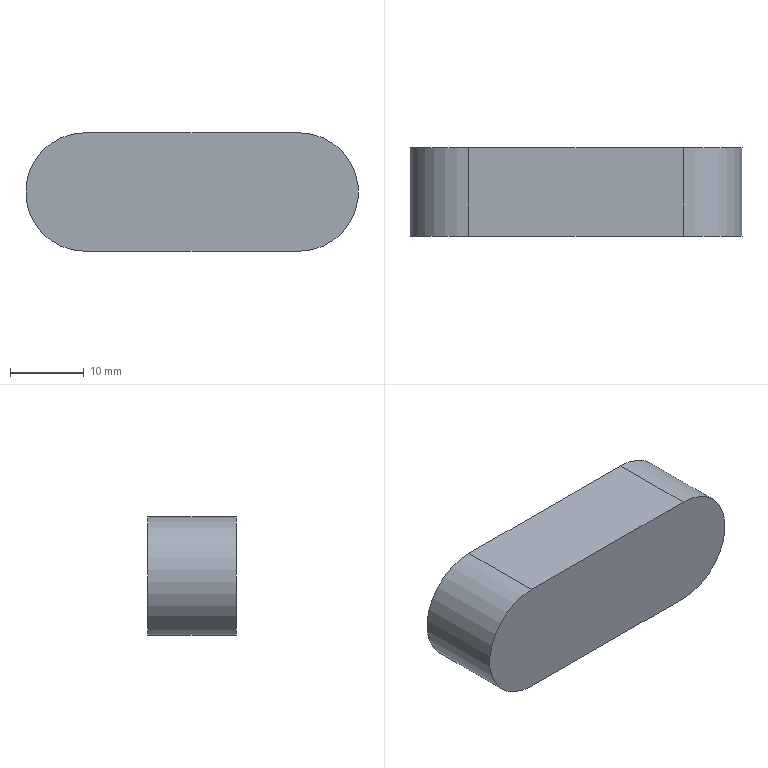Part | SolidWorks | features Extrusion 1 | 1 solid | 6 faces | box 45 x 12 x 16 mm | volume 7981 mm3 | plane 4 | cylinder 2 | commonest cylinder face diameters 16 x2
STEP:
#1=CARTESIAN_POINT('',(0.,0.,-8.));
#2=VERTEX_POINT('',#1);
#3=CARTESIAN_POINT('',(0.,0.,8.));
#4=VERTEX_POINT('',#3);
#5=CARTESIAN_POINT('',(0.,0.,0.));
#6=DIRECTION('',(0.,1.,0.));
#7=DIRECTION('',(0.,0.,1.));
#8=AXIS2_PLACEMENT_3D('',#5,#6,#7);
#9=CIRCLE('',#8,8.);
#10=EDGE_CURVE('',#2,#4,#9,.T.);
#11=ORIENTED_EDGE('',*,*,#10,.T.);
#12=CARTESIAN_POINT('',(0.,12.,8.));
#13=VERTEX_POINT('',#12);
#14=CARTESIAN_POINT('',(0.,12.,8.));
#15=DIRECTION('',(0.,-1.,0.));
#16=VECTOR('',#15,1000.);
#17=LINE('',#14,#16);
#18=EDGE_CURVE('',#13,#4,#17,.T.);
#19=ORIENTED_EDGE('',*,*,#18,.F.);
#20=CARTESIAN_POINT('',(0.,12.,-8.));
#21=VERTEX_POINT('',#20);
#22=CARTESIAN_POINT('',(0.,12.,0.));
#23=DIRECTION('',(0.,1.,0.));
#24=DIRECTION('',(0.,0.,1.));
#25=AXIS2_PLACEMENT_3D('',#22,#23,#24);
#26=CIRCLE('',#25,8.);
#27=EDGE_CURVE('',#21,#13,#26,.T.);
#28=ORIENTED_EDGE('',*,*,#27,.F.);
#29=CARTESIAN_POINT('',(0.,12.,-8.));
#30=DIRECTION('',(0.,-1.,0.));
#31=VECTOR('',#30,1000.);
#32=LINE('',#29,#31);
#33=EDGE_CURVE('',#21,#2,#32,.T.);
#34=ORIENTED_EDGE('',*,*,#33,.T.);
#35=EDGE_LOOP('',(#11,#19,#28,#34));
#36=FACE_OUTER_BOUND('',#35,.T.);
#37=CARTESIAN_POINT('',(0.,12.,0.));
#38=DIRECTION('',(0.,-1.,0.));
#39=DIRECTION('',(0.,0.,-1.));
#40=AXIS2_PLACEMENT_3D('',#37,#38,#39);
#41=CYLINDRICAL_SURFACE('',#40,8.);
#42=ADVANCED_FACE('',(#36),#41,.T.);
#43=CARTESIAN_POINT('',(29.,0.,8.));
#44=VERTEX_POINT('',#43);
#45=CARTESIAN_POINT('',(0.,0.,8.));
#46=DIRECTION('',(1.,0.,0.));
#47=VECTOR('',#46,1000.);
#48=LINE('',#45,#47);
#49=EDGE_CURVE('',#4,#44,#48,.T.);
#50=ORIENTED_EDGE('',*,*,#49,.T.);
#51=CARTESIAN_POINT('',(29.,12.,8.));
#52=VERTEX_POINT('',#51);
#53=CARTESIAN_POINT('',(29.,12.,8.));
#54=DIRECTION('',(0.,-1.,0.));
#55=VECTOR('',#54,1000.);
#56=LINE('',#53,#55);
#57=EDGE_CURVE('',#52,#44,#56,.T.);
#58=ORIENTED_EDGE('',*,*,#57,.F.);
#59=CARTESIAN_POINT('',(0.,12.,8.));
#60=DIRECTION('',(1.,0.,0.));
#61=VECTOR('',#60,1000.);
#62=LINE('',#59,#61);
#63=EDGE_CURVE('',#13,#52,#62,.T.);
#64=ORIENTED_EDGE('',*,*,#63,.F.);
#65=ORIENTED_EDGE('',*,*,#18,.T.);
#66=EDGE_LOOP('',(#50,#58,#64,#65));
#67=FACE_OUTER_BOUND('',#66,.T.);
#68=CARTESIAN_POINT('',(0.,12.,8.));
#69=DIRECTION('',(0.,0.,-1.));
#70=DIRECTION('',(-1.,0.,0.));
#71=AXIS2_PLACEMENT_3D('',#68,#69,#70);
#72=PLANE('',#71);
#73=ADVANCED_FACE('',(#67),#72,.F.);
#74=CARTESIAN_POINT('',(29.,0.,-8.));
#75=VERTEX_POINT('',#74);
#76=CARTESIAN_POINT('',(29.,0.,0.));
#77=DIRECTION('',(0.,1.,0.));
#78=DIRECTION('',(0.,0.,1.));
#79=AXIS2_PLACEMENT_3D('',#76,#77,#78);
#80=CIRCLE('',#79,8.);
#81=EDGE_CURVE('',#44,#75,#80,.T.);
#82=ORIENTED_EDGE('',*,*,#81,.T.);
#83=CARTESIAN_POINT('',(29.,12.,-8.));
#84=VERTEX_POINT('',#83);
#85=CARTESIAN_POINT('',(29.,12.,-8.));
#86=DIRECTION('',(0.,-1.,0.));
#87=VECTOR('',#86,1000.);
#88=LINE('',#85,#87);
#89=EDGE_CURVE('',#84,#75,#88,.T.);
#90=ORIENTED_EDGE('',*,*,#89,.F.);
#91=CARTESIAN_POINT('',(29.,12.,0.));
#92=DIRECTION('',(0.,1.,0.));
#93=DIRECTION('',(0.,0.,1.));
#94=AXIS2_PLACEMENT_3D('',#91,#92,#93);
#95=CIRCLE('',#94,8.);
#96=EDGE_CURVE('',#52,#84,#95,.T.);
#97=ORIENTED_EDGE('',*,*,#96,.F.);
#98=ORIENTED_EDGE('',*,*,#57,.T.);
#99=EDGE_LOOP('',(#82,#90,#97,#98));
#100=FACE_OUTER_BOUND('',#99,.T.);
#101=CARTESIAN_POINT('',(29.,12.,0.));
#102=DIRECTION('',(0.,-1.,0.));
#103=DIRECTION('',(0.,0.,-1.));
#104=AXIS2_PLACEMENT_3D('',#101,#102,#103);
#105=CYLINDRICAL_SURFACE('',#104,8.);
#106=ADVANCED_FACE('',(#100),#105,.T.);
#107=CARTESIAN_POINT('',(0.,0.,-8.));
#108=DIRECTION('',(-1.,0.,0.));
#109=VECTOR('',#108,1000.);
#110=LINE('',#107,#109);
#111=EDGE_CURVE('',#75,#2,#110,.T.);
#112=ORIENTED_EDGE('',*,*,#111,.T.);
#113=ORIENTED_EDGE('',*,*,#33,.F.);
#114=CARTESIAN_POINT('',(0.,12.,-8.));
#115=DIRECTION('',(-1.,0.,0.));
#116=VECTOR('',#115,1000.);
#117=LINE('',#114,#116);
#118=EDGE_CURVE('',#84,#21,#117,.T.);
#119=ORIENTED_EDGE('',*,*,#118,.F.);
#120=ORIENTED_EDGE('',*,*,#89,.T.);
#121=EDGE_LOOP('',(#112,#113,#119,#120));
#122=FACE_OUTER_BOUND('',#121,.T.);
#123=CARTESIAN_POINT('',(0.,12.,-8.));
#124=DIRECTION('',(0.,0.,1.));
#125=DIRECTION('',(1.,0.,0.));
#126=AXIS2_PLACEMENT_3D('',#123,#124,#125);
#127=PLANE('',#126);
#128=ADVANCED_FACE('',(#122),#127,.F.);
#129=ORIENTED_EDGE('',*,*,#27,.T.);
#130=ORIENTED_EDGE('',*,*,#63,.T.);
#131=ORIENTED_EDGE('',*,*,#96,.T.);
#132=ORIENTED_EDGE('',*,*,#118,.T.);
#133=EDGE_LOOP('',(#129,#130,#131,#132));
#134=FACE_OUTER_BOUND('',#133,.T.);
#135=CARTESIAN_POINT('',(0.,12.,0.));
#136=DIRECTION('',(0.,1.,0.));
#137=DIRECTION('',(0.,0.,1.));
#138=AXIS2_PLACEMENT_3D('',#135,#136,#137);
#139=PLANE('',#138);
#140=ADVANCED_FACE('',(#134),#139,.T.);
#141=ORIENTED_EDGE('',*,*,#10,.F.);
#142=ORIENTED_EDGE('',*,*,#111,.F.);
#143=ORIENTED_EDGE('',*,*,#81,.F.);
#144=ORIENTED_EDGE('',*,*,#49,.F.);
#145=EDGE_LOOP('',(#141,#142,#143,#144));
#146=FACE_OUTER_BOUND('',#145,.T.);
#147=CARTESIAN_POINT('',(0.,0.,0.));
#148=DIRECTION('',(0.,1.,0.));
#149=DIRECTION('',(0.,0.,1.));
#150=AXIS2_PLACEMENT_3D('',#147,#148,#149);
#151=PLANE('',#150);
#152=ADVANCED_FACE('',(#146),#151,.F.);
#153=CLOSED_SHELL('',(#42,#73,#106,#128,#140,#152));
#154=MANIFOLD_SOLID_BREP('',#153);
#155=CARTESIAN_POINT('',(0.,0.,0.));
#156=DIRECTION('',(0.,0.,1.));
#157=DIRECTION('',(1.,0.,0.));
#158=AXIS2_PLACEMENT_3D('',#155,#156,#157);
#159=(LENGTH_UNIT()NAMED_UNIT(*)SI_UNIT(.MILLI.,.METRE.));
#160=UNCERTAINTY_MEASURE_WITH_UNIT(LENGTH_MEASURE(0.00001),#159,'','');
#161=(NAMED_UNIT(*)PLANE_ANGLE_UNIT()SI_UNIT($,.RADIAN.));
#162=(NAMED_UNIT(*)SI_UNIT($,.STERADIAN.)SOLID_ANGLE_UNIT());
#163=(GEOMETRIC_REPRESENTATION_CONTEXT(3)GLOBAL_UNCERTAINTY_ASSIGNED_CONTEXT((#160))GLOBAL_UNIT_ASSIGNED_CONTEXT((#159,#161,#162))REPRESENTATION_CONTEXT('',''));
#164=ADVANCED_BREP_SHAPE_REPRESENTATION('',(#154,#158),#163);